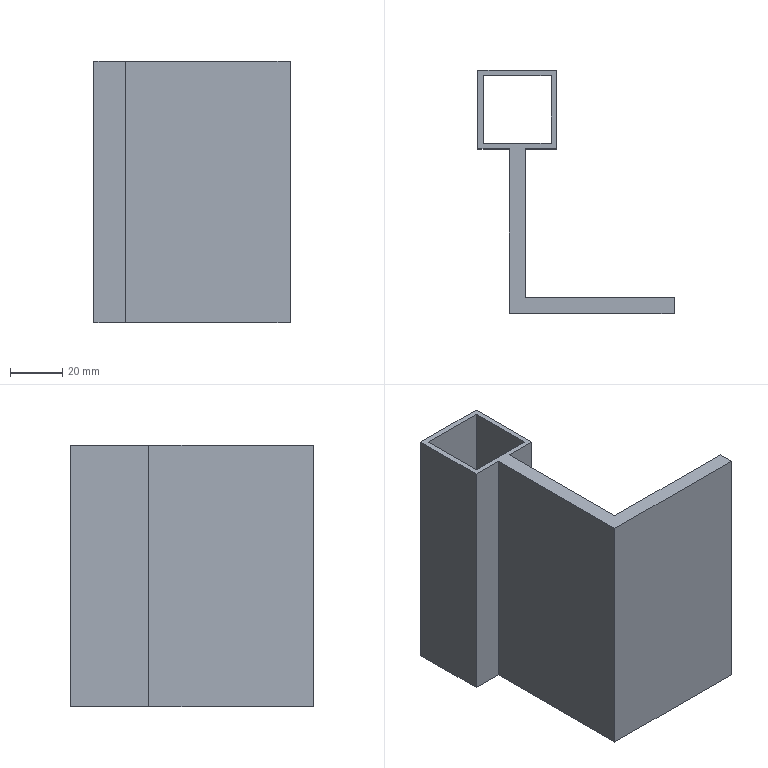Part | NX | features solid 2 | 1 solid | 16 faces | box 75 x 93 x 100 mm | volume 94400 mm3 | plane 16
STEP:
#1=CARTESIAN_POINT('',(-785.5,746.,-317.305));
#2=VERTEX_POINT('',#1);
#3=CARTESIAN_POINT('',(-728.5,746.,-317.305));
#4=VERTEX_POINT('',#3);
#5=CARTESIAN_POINT('',(-788.5,746.,-317.305));
#6=DIRECTION('',(1.,0.,0.));
#7=VECTOR('',#6,1000.);
#8=LINE('',#5,#7);
#9=EDGE_CURVE('',#2,#4,#8,.T.);
#10=ORIENTED_EDGE('',*,*,#9,.T.);
#11=CARTESIAN_POINT('',(-728.5,740.,-317.305));
#12=VERTEX_POINT('',#11);
#13=CARTESIAN_POINT('',(-728.5,743.,-317.305));
#14=DIRECTION('',(0.,1.,0.));
#15=VECTOR('',#14,1000.);
#16=LINE('',#13,#15);
#17=EDGE_CURVE('',#12,#4,#16,.T.);
#18=ORIENTED_EDGE('',*,*,#17,.F.);
#19=CARTESIAN_POINT('',(-791.5,740.,-317.305));
#20=VERTEX_POINT('',#19);
#21=CARTESIAN_POINT('',(-788.5,740.,-317.305));
#22=DIRECTION('',(1.,0.,0.));
#23=VECTOR('',#22,1000.);
#24=LINE('',#21,#23);
#25=EDGE_CURVE('',#20,#12,#24,.T.);
#26=ORIENTED_EDGE('',*,*,#25,.F.);
#27=CARTESIAN_POINT('',(-791.5,803.,-317.305));
#28=VERTEX_POINT('',#27);
#29=CARTESIAN_POINT('',(-791.5,743.,-317.305));
#30=DIRECTION('',(0.,1.,0.));
#31=VECTOR('',#30,1000.);
#32=LINE('',#29,#31);
#33=EDGE_CURVE('',#20,#28,#32,.T.);
#34=ORIENTED_EDGE('',*,*,#33,.T.);
#35=CARTESIAN_POINT('',(-803.5,803.,-317.305));
#36=VERTEX_POINT('',#35);
#37=CARTESIAN_POINT('',(-773.5,803.,-317.305));
#38=DIRECTION('',(-1.,0.,0.));
#39=VECTOR('',#38,1000.);
#40=LINE('',#37,#39);
#41=EDGE_CURVE('',#28,#36,#40,.T.);
#42=ORIENTED_EDGE('',*,*,#41,.T.);
#43=CARTESIAN_POINT('',(-803.5,833.,-317.305));
#44=VERTEX_POINT('',#43);
#45=CARTESIAN_POINT('',(-803.5,803.,-317.305));
#46=DIRECTION('',(0.,1.,0.));
#47=VECTOR('',#46,1000.);
#48=LINE('',#45,#47);
#49=EDGE_CURVE('',#36,#44,#48,.T.);
#50=ORIENTED_EDGE('',*,*,#49,.T.);
#51=CARTESIAN_POINT('',(-773.5,833.,-317.305));
#52=VERTEX_POINT('',#51);
#53=CARTESIAN_POINT('',(-803.5,833.,-317.305));
#54=DIRECTION('',(1.,0.,0.));
#55=VECTOR('',#54,1000.);
#56=LINE('',#53,#55);
#57=EDGE_CURVE('',#44,#52,#56,.T.);
#58=ORIENTED_EDGE('',*,*,#57,.T.);
#59=CARTESIAN_POINT('',(-773.5,803.,-317.305));
#60=VERTEX_POINT('',#59);
#61=CARTESIAN_POINT('',(-773.5,833.,-317.305));
#62=DIRECTION('',(0.,-1.,0.));
#63=VECTOR('',#62,1000.);
#64=LINE('',#61,#63);
#65=EDGE_CURVE('',#52,#60,#64,.T.);
#66=ORIENTED_EDGE('',*,*,#65,.T.);
#67=CARTESIAN_POINT('',(-785.5,803.,-317.305));
#68=VERTEX_POINT('',#67);
#69=CARTESIAN_POINT('',(-773.5,803.,-317.305));
#70=DIRECTION('',(-1.,0.,0.));
#71=VECTOR('',#70,1000.);
#72=LINE('',#69,#71);
#73=EDGE_CURVE('',#60,#68,#72,.T.);
#74=ORIENTED_EDGE('',*,*,#73,.T.);
#75=CARTESIAN_POINT('',(-785.5,743.,-317.305));
#76=DIRECTION('',(0.,1.,0.));
#77=VECTOR('',#76,1000.);
#78=LINE('',#75,#77);
#79=EDGE_CURVE('',#2,#68,#78,.T.);
#80=ORIENTED_EDGE('',*,*,#79,.F.);
#81=EDGE_LOOP('',(#10,#18,#26,#34,#42,#50,#58,#66,#74,#80));
#82=FACE_BOUND('',#81,.T.);
#83=CARTESIAN_POINT('',(-801.5,805.,-317.305));
#84=VERTEX_POINT('',#83);
#85=CARTESIAN_POINT('',(-801.5,831.,-317.305));
#86=VERTEX_POINT('',#85);
#87=CARTESIAN_POINT('',(-801.5,803.,-317.305));
#88=DIRECTION('',(0.,1.,0.));
#89=VECTOR('',#88,1000.);
#90=LINE('',#87,#89);
#91=EDGE_CURVE('',#84,#86,#90,.T.);
#92=ORIENTED_EDGE('',*,*,#91,.F.);
#93=CARTESIAN_POINT('',(-775.5,805.,-317.305));
#94=VERTEX_POINT('',#93);
#95=CARTESIAN_POINT('',(-773.5,805.,-317.305));
#96=DIRECTION('',(-1.,0.,0.));
#97=VECTOR('',#96,1000.);
#98=LINE('',#95,#97);
#99=EDGE_CURVE('',#94,#84,#98,.T.);
#100=ORIENTED_EDGE('',*,*,#99,.F.);
#101=CARTESIAN_POINT('',(-775.5,831.,-317.305));
#102=VERTEX_POINT('',#101);
#103=CARTESIAN_POINT('',(-775.5,833.,-317.305));
#104=DIRECTION('',(0.,-1.,0.));
#105=VECTOR('',#104,1000.);
#106=LINE('',#103,#105);
#107=EDGE_CURVE('',#102,#94,#106,.T.);
#108=ORIENTED_EDGE('',*,*,#107,.F.);
#109=CARTESIAN_POINT('',(-803.5,831.,-317.305));
#110=DIRECTION('',(1.,0.,0.));
#111=VECTOR('',#110,1000.);
#112=LINE('',#109,#111);
#113=EDGE_CURVE('',#86,#102,#112,.T.);
#114=ORIENTED_EDGE('',*,*,#113,.F.);
#115=EDGE_LOOP('',(#92,#100,#108,#114));
#116=FACE_BOUND('',#115,.T.);
#117=CARTESIAN_POINT('',(-788.5,743.,-317.305));
#118=DIRECTION('',(0.,0.,-1.));
#119=DIRECTION('',(1.,0.,0.));
#120=AXIS2_PLACEMENT_3D('',#117,#118,#119);
#121=PLANE('',#120);
#122=ADVANCED_FACE('',(#82,#116),#121,.T.);
#123=ORIENTED_EDGE('',*,*,#17,.T.);
#124=CARTESIAN_POINT('',(-728.5,746.,-217.305));
#125=VERTEX_POINT('',#124);
#126=CARTESIAN_POINT('',(-728.5,746.,-317.305));
#127=DIRECTION('',(0.,0.,-1.));
#128=VECTOR('',#127,1000.);
#129=LINE('',#126,#128);
#130=EDGE_CURVE('',#4,#125,#129,.F.);
#131=ORIENTED_EDGE('',*,*,#130,.T.);
#132=CARTESIAN_POINT('',(-728.5,740.,-217.305));
#133=VERTEX_POINT('',#132);
#134=CARTESIAN_POINT('',(-728.5,743.,-217.305));
#135=DIRECTION('',(0.,1.,0.));
#136=VECTOR('',#135,1000.);
#137=LINE('',#134,#136);
#138=EDGE_CURVE('',#133,#125,#137,.T.);
#139=ORIENTED_EDGE('',*,*,#138,.F.);
#140=CARTESIAN_POINT('',(-728.5,740.,-317.305));
#141=DIRECTION('',(0.,0.,-1.));
#142=VECTOR('',#141,1000.);
#143=LINE('',#140,#142);
#144=EDGE_CURVE('',#12,#133,#143,.F.);
#145=ORIENTED_EDGE('',*,*,#144,.F.);
#146=EDGE_LOOP('',(#123,#131,#139,#145));
#147=FACE_BOUND('',#146,.T.);
#148=CARTESIAN_POINT('',(-728.5,743.,-317.305));
#149=DIRECTION('',(1.,0.,0.));
#150=DIRECTION('',(0.,0.,1.));
#151=AXIS2_PLACEMENT_3D('',#148,#149,#150);
#152=PLANE('',#151);
#153=ADVANCED_FACE('',(#147),#152,.T.);
#154=CARTESIAN_POINT('',(-785.5,746.,-217.305));
#155=VERTEX_POINT('',#154);
#156=CARTESIAN_POINT('',(-785.5,803.,-217.305));
#157=VERTEX_POINT('',#156);
#158=CARTESIAN_POINT('',(-785.5,743.,-217.305));
#159=DIRECTION('',(0.,1.,0.));
#160=VECTOR('',#159,1000.);
#161=LINE('',#158,#160);
#162=EDGE_CURVE('',#155,#157,#161,.T.);
#163=ORIENTED_EDGE('',*,*,#162,.T.);
#164=CARTESIAN_POINT('',(-773.5,803.,-217.305));
#165=VERTEX_POINT('',#164);
#166=CARTESIAN_POINT('',(-773.5,803.,-217.305));
#167=DIRECTION('',(-1.,0.,0.));
#168=VECTOR('',#167,1000.);
#169=LINE('',#166,#168);
#170=EDGE_CURVE('',#165,#157,#169,.T.);
#171=ORIENTED_EDGE('',*,*,#170,.F.);
#172=CARTESIAN_POINT('',(-773.5,833.,-217.305));
#173=VERTEX_POINT('',#172);
#174=CARTESIAN_POINT('',(-773.5,833.,-217.305));
#175=DIRECTION('',(0.,-1.,0.));
#176=VECTOR('',#175,1000.);
#177=LINE('',#174,#176);
#178=EDGE_CURVE('',#173,#165,#177,.T.);
#179=ORIENTED_EDGE('',*,*,#178,.F.);
#180=CARTESIAN_POINT('',(-803.5,833.,-217.305));
#181=VERTEX_POINT('',#180);
#182=CARTESIAN_POINT('',(-803.5,833.,-217.305));
#183=DIRECTION('',(1.,0.,0.));
#184=VECTOR('',#183,1000.);
#185=LINE('',#182,#184);
#186=EDGE_CURVE('',#181,#173,#185,.T.);
#187=ORIENTED_EDGE('',*,*,#186,.F.);
#188=CARTESIAN_POINT('',(-803.5,803.,-217.305));
#189=VERTEX_POINT('',#188);
#190=CARTESIAN_POINT('',(-803.5,803.,-217.305));
#191=DIRECTION('',(0.,1.,0.));
#192=VECTOR('',#191,1000.);
#193=LINE('',#190,#192);
#194=EDGE_CURVE('',#189,#181,#193,.T.);
#195=ORIENTED_EDGE('',*,*,#194,.F.);
#196=CARTESIAN_POINT('',(-791.5,803.,-217.305));
#197=VERTEX_POINT('',#196);
#198=CARTESIAN_POINT('',(-773.5,803.,-217.305));
#199=DIRECTION('',(-1.,0.,0.));
#200=VECTOR('',#199,1000.);
#201=LINE('',#198,#200);
#202=EDGE_CURVE('',#197,#189,#201,.T.);
#203=ORIENTED_EDGE('',*,*,#202,.F.);
#204=CARTESIAN_POINT('',(-791.5,740.,-217.305));
#205=VERTEX_POINT('',#204);
#206=CARTESIAN_POINT('',(-791.5,743.,-217.305));
#207=DIRECTION('',(0.,1.,0.));
#208=VECTOR('',#207,1000.);
#209=LINE('',#206,#208);
#210=EDGE_CURVE('',#205,#197,#209,.T.);
#211=ORIENTED_EDGE('',*,*,#210,.F.);
#212=CARTESIAN_POINT('',(-788.5,740.,-217.305));
#213=DIRECTION('',(1.,0.,0.));
#214=VECTOR('',#213,1000.);
#215=LINE('',#212,#214);
#216=EDGE_CURVE('',#205,#133,#215,.T.);
#217=ORIENTED_EDGE('',*,*,#216,.T.);
#218=ORIENTED_EDGE('',*,*,#138,.T.);
#219=CARTESIAN_POINT('',(-788.5,746.,-217.305));
#220=DIRECTION('',(1.,0.,0.));
#221=VECTOR('',#220,1000.);
#222=LINE('',#219,#221);
#223=EDGE_CURVE('',#155,#125,#222,.T.);
#224=ORIENTED_EDGE('',*,*,#223,.F.);
#225=EDGE_LOOP('',(#163,#171,#179,#187,#195,#203,#211,#217,#218,#224));
#226=FACE_BOUND('',#225,.T.);
#227=CARTESIAN_POINT('',(-801.5,805.,-217.305));
#228=VERTEX_POINT('',#227);
#229=CARTESIAN_POINT('',(-801.5,831.,-217.305));
#230=VERTEX_POINT('',#229);
#231=CARTESIAN_POINT('',(-801.5,803.,-217.305));
#232=DIRECTION('',(0.,1.,0.));
#233=VECTOR('',#232,1000.);
#234=LINE('',#231,#233);
#235=EDGE_CURVE('',#228,#230,#234,.T.);
#236=ORIENTED_EDGE('',*,*,#235,.T.);
#237=CARTESIAN_POINT('',(-775.5,831.,-217.305));
#238=VERTEX_POINT('',#237);
#239=CARTESIAN_POINT('',(-803.5,831.,-217.305));
#240=DIRECTION('',(1.,0.,0.));
#241=VECTOR('',#240,1000.);
#242=LINE('',#239,#241);
#243=EDGE_CURVE('',#230,#238,#242,.T.);
#244=ORIENTED_EDGE('',*,*,#243,.T.);
#245=CARTESIAN_POINT('',(-775.5,805.,-217.305));
#246=VERTEX_POINT('',#245);
#247=CARTESIAN_POINT('',(-775.5,833.,-217.305));
#248=DIRECTION('',(0.,-1.,0.));
#249=VECTOR('',#248,1000.);
#250=LINE('',#247,#249);
#251=EDGE_CURVE('',#238,#246,#250,.T.);
#252=ORIENTED_EDGE('',*,*,#251,.T.);
#253=CARTESIAN_POINT('',(-773.5,805.,-217.305));
#254=DIRECTION('',(-1.,0.,0.));
#255=VECTOR('',#254,1000.);
#256=LINE('',#253,#255);
#257=EDGE_CURVE('',#246,#228,#256,.T.);
#258=ORIENTED_EDGE('',*,*,#257,.T.);
#259=EDGE_LOOP('',(#236,#244,#252,#258));
#260=FACE_BOUND('',#259,.T.);
#261=CARTESIAN_POINT('',(-788.5,743.,-217.305));
#262=DIRECTION('',(0.,0.,-1.));
#263=DIRECTION('',(0.,1.,0.));
#264=AXIS2_PLACEMENT_3D('',#261,#262,#263);
#265=PLANE('',#264);
#266=ADVANCED_FACE('',(#226,#260),#265,.F.);
#267=ORIENTED_EDGE('',*,*,#162,.F.);
#268=CARTESIAN_POINT('',(-785.5,746.,-317.305));
#269=DIRECTION('',(0.,0.,1.));
#270=VECTOR('',#269,1000.);
#271=LINE('',#268,#270);
#272=EDGE_CURVE('',#2,#155,#271,.T.);
#273=ORIENTED_EDGE('',*,*,#272,.F.);
#274=ORIENTED_EDGE('',*,*,#79,.T.);
#275=CARTESIAN_POINT('',(-785.5,803.,-317.305));
#276=DIRECTION('',(0.,0.,1.));
#277=VECTOR('',#276,1000.);
#278=LINE('',#275,#277);
#279=EDGE_CURVE('',#68,#157,#278,.T.);
#280=ORIENTED_EDGE('',*,*,#279,.T.);
#281=EDGE_LOOP('',(#267,#273,#274,#280));
#282=FACE_BOUND('',#281,.T.);
#283=CARTESIAN_POINT('',(-785.5,743.,-317.305));
#284=DIRECTION('',(-1.,0.,0.));
#285=DIRECTION('',(0.,1.,0.));
#286=AXIS2_PLACEMENT_3D('',#283,#284,#285);
#287=PLANE('',#286);
#288=ADVANCED_FACE('',(#282),#287,.F.);
#289=ORIENTED_EDGE('',*,*,#223,.T.);
#290=ORIENTED_EDGE('',*,*,#130,.F.);
#291=ORIENTED_EDGE('',*,*,#9,.F.);
#292=ORIENTED_EDGE('',*,*,#272,.T.);
#293=EDGE_LOOP('',(#289,#290,#291,#292));
#294=FACE_BOUND('',#293,.T.);
#295=CARTESIAN_POINT('',(-788.5,746.,-317.305));
#296=DIRECTION('',(0.,1.,0.));
#297=DIRECTION('',(0.,0.,-1.));
#298=AXIS2_PLACEMENT_3D('',#295,#296,#297);
#299=PLANE('',#298);
#300=ADVANCED_FACE('',(#294),#299,.T.);
#301=ORIENTED_EDGE('',*,*,#210,.T.);
#302=CARTESIAN_POINT('',(-791.5,803.,-317.305));
#303=DIRECTION('',(0.,0.,1.));
#304=VECTOR('',#303,1000.);
#305=LINE('',#302,#304);
#306=EDGE_CURVE('',#28,#197,#305,.T.);
#307=ORIENTED_EDGE('',*,*,#306,.F.);
#308=ORIENTED_EDGE('',*,*,#33,.F.);
#309=CARTESIAN_POINT('',(-791.5,740.,-317.305));
#310=DIRECTION('',(0.,0.,1.));
#311=VECTOR('',#310,1000.);
#312=LINE('',#309,#311);
#313=EDGE_CURVE('',#20,#205,#312,.T.);
#314=ORIENTED_EDGE('',*,*,#313,.T.);
#315=EDGE_LOOP('',(#301,#307,#308,#314));
#316=FACE_BOUND('',#315,.T.);
#317=CARTESIAN_POINT('',(-791.5,743.,-317.305));
#318=DIRECTION('',(-1.,0.,0.));
#319=DIRECTION('',(0.,1.,0.));
#320=AXIS2_PLACEMENT_3D('',#317,#318,#319);
#321=PLANE('',#320);
#322=ADVANCED_FACE('',(#316),#321,.T.);
#323=ORIENTED_EDGE('',*,*,#216,.F.);
#324=ORIENTED_EDGE('',*,*,#313,.F.);
#325=ORIENTED_EDGE('',*,*,#25,.T.);
#326=ORIENTED_EDGE('',*,*,#144,.T.);
#327=EDGE_LOOP('',(#323,#324,#325,#326));
#328=FACE_BOUND('',#327,.T.);
#329=CARTESIAN_POINT('',(-788.5,740.,-317.305));
#330=DIRECTION('',(0.,1.,0.));
#331=DIRECTION('',(0.,0.,-1.));
#332=AXIS2_PLACEMENT_3D('',#329,#330,#331);
#333=PLANE('',#332);
#334=ADVANCED_FACE('',(#328),#333,.F.);
#335=ORIENTED_EDGE('',*,*,#306,.T.);
#336=ORIENTED_EDGE('',*,*,#202,.T.);
#337=CARTESIAN_POINT('',(-803.5,803.,-317.305));
#338=DIRECTION('',(0.,0.,1.));
#339=VECTOR('',#338,1000.);
#340=LINE('',#337,#339);
#341=EDGE_CURVE('',#36,#189,#340,.T.);
#342=ORIENTED_EDGE('',*,*,#341,.F.);
#343=ORIENTED_EDGE('',*,*,#41,.F.);
#344=EDGE_LOOP('',(#335,#336,#342,#343));
#345=FACE_BOUND('',#344,.T.);
#346=CARTESIAN_POINT('',(-773.5,803.,-317.305));
#347=DIRECTION('',(0.,-1.,0.));
#348=DIRECTION('',(-1.,0.,0.));
#349=AXIS2_PLACEMENT_3D('',#346,#347,#348);
#350=PLANE('',#349);
#351=ADVANCED_FACE('',(#345),#350,.T.);
#352=ORIENTED_EDGE('',*,*,#235,.F.);
#353=CARTESIAN_POINT('',(-801.5,805.,-317.305));
#354=DIRECTION('',(0.,0.,1.));
#355=VECTOR('',#354,1000.);
#356=LINE('',#353,#355);
#357=EDGE_CURVE('',#84,#228,#356,.T.);
#358=ORIENTED_EDGE('',*,*,#357,.F.);
#359=ORIENTED_EDGE('',*,*,#91,.T.);
#360=CARTESIAN_POINT('',(-801.5,831.,-317.305));
#361=DIRECTION('',(0.,0.,1.));
#362=VECTOR('',#361,1000.);
#363=LINE('',#360,#362);
#364=EDGE_CURVE('',#86,#230,#363,.T.);
#365=ORIENTED_EDGE('',*,*,#364,.T.);
#366=EDGE_LOOP('',(#352,#358,#359,#365));
#367=FACE_BOUND('',#366,.T.);
#368=CARTESIAN_POINT('',(-801.5,803.,-317.305));
#369=DIRECTION('',(-1.,0.,0.));
#370=DIRECTION('',(0.,1.,0.));
#371=AXIS2_PLACEMENT_3D('',#368,#369,#370);
#372=PLANE('',#371);
#373=ADVANCED_FACE('',(#367),#372,.F.);
#374=ORIENTED_EDGE('',*,*,#243,.F.);
#375=ORIENTED_EDGE('',*,*,#364,.F.);
#376=ORIENTED_EDGE('',*,*,#113,.T.);
#377=CARTESIAN_POINT('',(-775.5,831.,-317.305));
#378=DIRECTION('',(0.,0.,1.));
#379=VECTOR('',#378,1000.);
#380=LINE('',#377,#379);
#381=EDGE_CURVE('',#102,#238,#380,.T.);
#382=ORIENTED_EDGE('',*,*,#381,.T.);
#383=EDGE_LOOP('',(#374,#375,#376,#382));
#384=FACE_BOUND('',#383,.T.);
#385=CARTESIAN_POINT('',(-803.5,831.,-317.305));
#386=DIRECTION('',(0.,1.,0.));
#387=DIRECTION('',(1.,0.,0.));
#388=AXIS2_PLACEMENT_3D('',#385,#386,#387);
#389=PLANE('',#388);
#390=ADVANCED_FACE('',(#384),#389,.F.);
#391=ORIENTED_EDGE('',*,*,#251,.F.);
#392=ORIENTED_EDGE('',*,*,#381,.F.);
#393=ORIENTED_EDGE('',*,*,#107,.T.);
#394=CARTESIAN_POINT('',(-775.5,805.,-317.305));
#395=DIRECTION('',(0.,0.,1.));
#396=VECTOR('',#395,1000.);
#397=LINE('',#394,#396);
#398=EDGE_CURVE('',#94,#246,#397,.T.);
#399=ORIENTED_EDGE('',*,*,#398,.T.);
#400=EDGE_LOOP('',(#391,#392,#393,#399));
#401=FACE_BOUND('',#400,.T.);
#402=CARTESIAN_POINT('',(-775.5,833.,-317.305));
#403=DIRECTION('',(1.,0.,0.));
#404=DIRECTION('',(0.,-1.,0.));
#405=AXIS2_PLACEMENT_3D('',#402,#403,#404);
#406=PLANE('',#405);
#407=ADVANCED_FACE('',(#401),#406,.F.);
#408=ORIENTED_EDGE('',*,*,#257,.F.);
#409=ORIENTED_EDGE('',*,*,#398,.F.);
#410=ORIENTED_EDGE('',*,*,#99,.T.);
#411=ORIENTED_EDGE('',*,*,#357,.T.);
#412=EDGE_LOOP('',(#408,#409,#410,#411));
#413=FACE_BOUND('',#412,.T.);
#414=CARTESIAN_POINT('',(-773.5,805.,-317.305));
#415=DIRECTION('',(0.,-1.,0.));
#416=DIRECTION('',(-1.,0.,0.));
#417=AXIS2_PLACEMENT_3D('',#414,#415,#416);
#418=PLANE('',#417);
#419=ADVANCED_FACE('',(#413),#418,.F.);
#420=ORIENTED_EDGE('',*,*,#194,.T.);
#421=CARTESIAN_POINT('',(-803.5,833.,-317.305));
#422=DIRECTION('',(0.,0.,1.));
#423=VECTOR('',#422,1000.);
#424=LINE('',#421,#423);
#425=EDGE_CURVE('',#44,#181,#424,.T.);
#426=ORIENTED_EDGE('',*,*,#425,.F.);
#427=ORIENTED_EDGE('',*,*,#49,.F.);
#428=ORIENTED_EDGE('',*,*,#341,.T.);
#429=EDGE_LOOP('',(#420,#426,#427,#428));
#430=FACE_BOUND('',#429,.T.);
#431=CARTESIAN_POINT('',(-803.5,803.,-317.305));
#432=DIRECTION('',(-1.,0.,0.));
#433=DIRECTION('',(0.,1.,0.));
#434=AXIS2_PLACEMENT_3D('',#431,#432,#433);
#435=PLANE('',#434);
#436=ADVANCED_FACE('',(#430),#435,.T.);
#437=ORIENTED_EDGE('',*,*,#186,.T.);
#438=CARTESIAN_POINT('',(-773.5,833.,-317.305));
#439=DIRECTION('',(0.,0.,1.));
#440=VECTOR('',#439,1000.);
#441=LINE('',#438,#440);
#442=EDGE_CURVE('',#52,#173,#441,.T.);
#443=ORIENTED_EDGE('',*,*,#442,.F.);
#444=ORIENTED_EDGE('',*,*,#57,.F.);
#445=ORIENTED_EDGE('',*,*,#425,.T.);
#446=EDGE_LOOP('',(#437,#443,#444,#445));
#447=FACE_BOUND('',#446,.T.);
#448=CARTESIAN_POINT('',(-803.5,833.,-317.305));
#449=DIRECTION('',(0.,1.,0.));
#450=DIRECTION('',(1.,0.,0.));
#451=AXIS2_PLACEMENT_3D('',#448,#449,#450);
#452=PLANE('',#451);
#453=ADVANCED_FACE('',(#447),#452,.T.);
#454=ORIENTED_EDGE('',*,*,#178,.T.);
#455=CARTESIAN_POINT('',(-773.5,803.,-317.305));
#456=DIRECTION('',(0.,0.,1.));
#457=VECTOR('',#456,1000.);
#458=LINE('',#455,#457);
#459=EDGE_CURVE('',#60,#165,#458,.T.);
#460=ORIENTED_EDGE('',*,*,#459,.F.);
#461=ORIENTED_EDGE('',*,*,#65,.F.);
#462=ORIENTED_EDGE('',*,*,#442,.T.);
#463=EDGE_LOOP('',(#454,#460,#461,#462));
#464=FACE_BOUND('',#463,.T.);
#465=CARTESIAN_POINT('',(-773.5,833.,-317.305));
#466=DIRECTION('',(1.,0.,0.));
#467=DIRECTION('',(0.,-1.,0.));
#468=AXIS2_PLACEMENT_3D('',#465,#466,#467);
#469=PLANE('',#468);
#470=ADVANCED_FACE('',(#464),#469,.T.);
#471=ORIENTED_EDGE('',*,*,#73,.F.);
#472=ORIENTED_EDGE('',*,*,#459,.T.);
#473=ORIENTED_EDGE('',*,*,#170,.T.);
#474=ORIENTED_EDGE('',*,*,#279,.F.);
#475=EDGE_LOOP('',(#471,#472,#473,#474));
#476=FACE_BOUND('',#475,.T.);
#477=CARTESIAN_POINT('',(-773.5,803.,-317.305));
#478=DIRECTION('',(0.,-1.,0.));
#479=DIRECTION('',(-1.,0.,0.));
#480=AXIS2_PLACEMENT_3D('',#477,#478,#479);
#481=PLANE('',#480);
#482=ADVANCED_FACE('',(#476),#481,.T.);
#483=CLOSED_SHELL('',(#122,#153,#266,#288,#300,#322,#334,#351,#373,#390,#407,#419,#436,#453,#470,#482));
#484=MANIFOLD_SOLID_BREP('',#483);
#485=(LENGTH_UNIT()NAMED_UNIT(*)SI_UNIT(.MILLI.,.METRE.));
#486=UNCERTAINTY_MEASURE_WITH_UNIT(LENGTH_MEASURE(0.00001),#485,'','');
#487=(NAMED_UNIT(*)PLANE_ANGLE_UNIT()SI_UNIT($,.RADIAN.));
#488=(NAMED_UNIT(*)SI_UNIT($,.STERADIAN.)SOLID_ANGLE_UNIT());
#489=(GEOMETRIC_REPRESENTATION_CONTEXT(3)GLOBAL_UNCERTAINTY_ASSIGNED_CONTEXT((#486))GLOBAL_UNIT_ASSIGNED_CONTEXT((#485,#487,#488))REPRESENTATION_CONTEXT('',''));
#490=ADVANCED_BREP_SHAPE_REPRESENTATION('',(#484),#489);